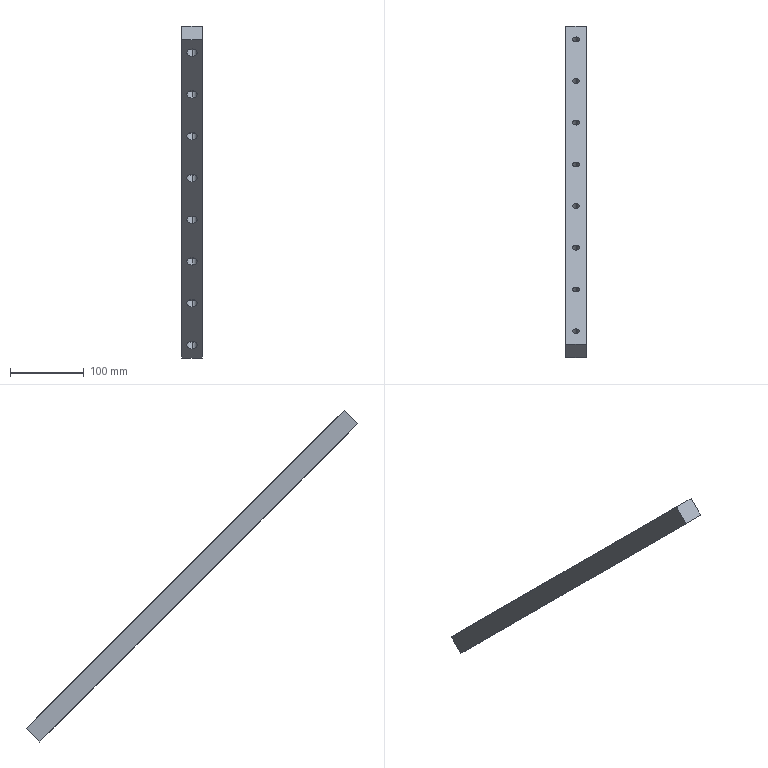Part | STEP file | X-Axis 28 Guide Rail | 1 solid | 46 faces | box 28 x 449.72 x 449.72 mm | volume 422177 mm3 | cylinder 32 | plane 14 | commonest cylinder face diameters 9 x16 14 x16
STEP:
#1=CARTESIAN_POINT('',(-773.,626.059,-470.164));
#2=VERTEX_POINT('',#1);
#3=CARTESIAN_POINT('',(-773.,632.423,-476.527));
#4=VERTEX_POINT('',#3);
#5=CARTESIAN_POINT('',(-773.,629.241,-473.346));
#6=DIRECTION('',(0.,-0.7071,-0.7071));
#7=DIRECTION('',(0.,0.7071,-0.7071));
#8=AXIS2_PLACEMENT_3D('',#5,#6,#7);
#9=CIRCLE('',#8,4.5);
#10=EDGE_CURVE('',#2,#4,#9,.T.);
#11=ORIENTED_EDGE('',*,*,#10,.F.);
#12=CARTESIAN_POINT('',(-773.,616.16,-480.063));
#13=VERTEX_POINT('',#12);
#14=CARTESIAN_POINT('',(-773.,607.674,-488.548));
#15=DIRECTION('',(0.,-0.7071,-0.7071));
#16=VECTOR('',#15,1000.);
#17=LINE('',#14,#16);
#18=EDGE_CURVE('',#2,#13,#17,.T.);
#19=ORIENTED_EDGE('',*,*,#18,.T.);
#20=CARTESIAN_POINT('',(-773.,622.524,-486.427));
#21=VERTEX_POINT('',#20);
#22=CARTESIAN_POINT('',(-773.,619.342,-483.245));
#23=DIRECTION('',(0.,0.7071,0.7071));
#24=DIRECTION('',(0.,0.7071,-0.7071));
#25=AXIS2_PLACEMENT_3D('',#22,#23,#24);
#26=CIRCLE('',#25,4.5);
#27=EDGE_CURVE('',#21,#13,#26,.T.);
#28=ORIENTED_EDGE('',*,*,#27,.F.);
#29=CARTESIAN_POINT('',(-773.,614.038,-494.912));
#30=DIRECTION('',(0.,-0.7071,-0.7071));
#31=VECTOR('',#30,1000.);
#32=LINE('',#29,#31);
#33=EDGE_CURVE('',#4,#21,#32,.T.);
#34=ORIENTED_EDGE('',*,*,#33,.F.);
#35=EDGE_LOOP('',(#11,#19,#28,#34));
#36=FACE_OUTER_BOUND('',#35,.T.);
#37=CARTESIAN_POINT('',(-773.,610.856,-491.73));
#38=DIRECTION('',(0.,-0.7071,-0.7071));
#39=DIRECTION('',(0.,0.7071,-0.7071));
#40=AXIS2_PLACEMENT_3D('',#37,#38,#39);
#41=CYLINDRICAL_SURFACE('',#40,4.5);
#42=ADVANCED_FACE('',(#36),#41,.F.);
#43=CARTESIAN_POINT('',(-773.,682.628,-526.732));
#44=VERTEX_POINT('',#43);
#45=CARTESIAN_POINT('',(-773.,688.992,-533.096));
#46=VERTEX_POINT('',#45);
#47=CARTESIAN_POINT('',(-773.,685.81,-529.914));
#48=DIRECTION('',(0.,-0.7071,-0.7071));
#49=DIRECTION('',(0.,0.7071,-0.7071));
#50=AXIS2_PLACEMENT_3D('',#47,#48,#49);
#51=CIRCLE('',#50,4.5);
#52=EDGE_CURVE('',#44,#46,#51,.T.);
#53=ORIENTED_EDGE('',*,*,#52,.F.);
#54=CARTESIAN_POINT('',(-773.,672.728,-536.632));
#55=VERTEX_POINT('',#54);
#56=CARTESIAN_POINT('',(-773.,664.243,-545.117));
#57=DIRECTION('',(0.,-0.7071,-0.7071));
#58=VECTOR('',#57,1000.);
#59=LINE('',#56,#58);
#60=EDGE_CURVE('',#44,#55,#59,.T.);
#61=ORIENTED_EDGE('',*,*,#60,.T.);
#62=CARTESIAN_POINT('',(-773.,679.092,-542.996));
#63=VERTEX_POINT('',#62);
#64=CARTESIAN_POINT('',(-773.,675.91,-539.814));
#65=DIRECTION('',(0.,0.7071,0.7071));
#66=DIRECTION('',(0.,0.7071,-0.7071));
#67=AXIS2_PLACEMENT_3D('',#64,#65,#66);
#68=CIRCLE('',#67,4.5);
#69=EDGE_CURVE('',#63,#55,#68,.T.);
#70=ORIENTED_EDGE('',*,*,#69,.F.);
#71=CARTESIAN_POINT('',(-773.,670.607,-551.481));
#72=DIRECTION('',(0.,-0.7071,-0.7071));
#73=VECTOR('',#72,1000.);
#74=LINE('',#71,#73);
#75=EDGE_CURVE('',#46,#63,#74,.T.);
#76=ORIENTED_EDGE('',*,*,#75,.F.);
#77=EDGE_LOOP('',(#53,#61,#70,#76));
#78=FACE_OUTER_BOUND('',#77,.T.);
#79=CARTESIAN_POINT('',(-773.,667.425,-548.299));
#80=DIRECTION('',(0.,-0.7071,-0.7071));
#81=DIRECTION('',(0.,0.7071,-0.7071));
#82=AXIS2_PLACEMENT_3D('',#79,#80,#81);
#83=CYLINDRICAL_SURFACE('',#82,4.5);
#84=ADVANCED_FACE('',(#78),#83,.F.);
#85=CARTESIAN_POINT('',(-773.,456.354,-300.458));
#86=VERTEX_POINT('',#85);
#87=CARTESIAN_POINT('',(-773.,462.717,-306.822));
#88=VERTEX_POINT('',#87);
#89=CARTESIAN_POINT('',(-773.,459.536,-303.64));
#90=DIRECTION('',(0.,-0.7071,-0.7071));
#91=DIRECTION('',(0.,0.7071,-0.7071));
#92=AXIS2_PLACEMENT_3D('',#89,#90,#91);
#93=CIRCLE('',#92,4.5);
#94=EDGE_CURVE('',#86,#88,#93,.T.);
#95=ORIENTED_EDGE('',*,*,#94,.F.);
#96=CARTESIAN_POINT('',(-773.,446.454,-310.357));
#97=VERTEX_POINT('',#96);
#98=CARTESIAN_POINT('',(-773.,437.969,-318.843));
#99=DIRECTION('',(0.,-0.7071,-0.7071));
#100=VECTOR('',#99,1000.);
#101=LINE('',#98,#100);
#102=EDGE_CURVE('',#86,#97,#101,.T.);
#103=ORIENTED_EDGE('',*,*,#102,.T.);
#104=CARTESIAN_POINT('',(-773.,452.818,-316.721));
#105=VERTEX_POINT('',#104);
#106=CARTESIAN_POINT('',(-773.,449.636,-313.539));
#107=DIRECTION('',(0.,0.7071,0.7071));
#108=DIRECTION('',(0.,0.7071,-0.7071));
#109=AXIS2_PLACEMENT_3D('',#106,#107,#108);
#110=CIRCLE('',#109,4.5);
#111=EDGE_CURVE('',#105,#97,#110,.T.);
#112=ORIENTED_EDGE('',*,*,#111,.F.);
#113=CARTESIAN_POINT('',(-773.,444.333,-325.207));
#114=DIRECTION('',(0.,-0.7071,-0.7071));
#115=VECTOR('',#114,1000.);
#116=LINE('',#113,#115);
#117=EDGE_CURVE('',#88,#105,#116,.T.);
#118=ORIENTED_EDGE('',*,*,#117,.F.);
#119=EDGE_LOOP('',(#95,#103,#112,#118));
#120=FACE_OUTER_BOUND('',#119,.T.);
#121=CARTESIAN_POINT('',(-773.,441.151,-322.025));
#122=DIRECTION('',(0.,-0.7071,-0.7071));
#123=DIRECTION('',(0.,0.7071,-0.7071));
#124=AXIS2_PLACEMENT_3D('',#121,#122,#123);
#125=CYLINDRICAL_SURFACE('',#124,4.5);
#126=ADVANCED_FACE('',(#120),#125,.F.);
#127=CARTESIAN_POINT('',(-773.,569.491,-413.595));
#128=VERTEX_POINT('',#127);
#129=CARTESIAN_POINT('',(-773.,575.855,-419.959));
#130=VERTEX_POINT('',#129);
#131=CARTESIAN_POINT('',(-773.,572.673,-416.777));
#132=DIRECTION('',(0.,-0.7071,-0.7071));
#133=DIRECTION('',(0.,0.7071,-0.7071));
#134=AXIS2_PLACEMENT_3D('',#131,#132,#133);
#135=CIRCLE('',#134,4.5);
#136=EDGE_CURVE('',#128,#130,#135,.T.);
#137=ORIENTED_EDGE('',*,*,#136,.F.);
#138=CARTESIAN_POINT('',(-773.,559.591,-423.494));
#139=VERTEX_POINT('',#138);
#140=CARTESIAN_POINT('',(-773.,551.106,-431.98));
#141=DIRECTION('',(0.,-0.7071,-0.7071));
#142=VECTOR('',#141,1000.);
#143=LINE('',#140,#142);
#144=EDGE_CURVE('',#128,#139,#143,.T.);
#145=ORIENTED_EDGE('',*,*,#144,.T.);
#146=CARTESIAN_POINT('',(-773.,565.955,-429.858));
#147=VERTEX_POINT('',#146);
#148=CARTESIAN_POINT('',(-773.,562.773,-426.676));
#149=DIRECTION('',(0.,0.7071,0.7071));
#150=DIRECTION('',(0.,0.7071,-0.7071));
#151=AXIS2_PLACEMENT_3D('',#148,#149,#150);
#152=CIRCLE('',#151,4.5);
#153=EDGE_CURVE('',#147,#139,#152,.T.);
#154=ORIENTED_EDGE('',*,*,#153,.F.);
#155=CARTESIAN_POINT('',(-773.,557.47,-438.344));
#156=DIRECTION('',(0.,-0.7071,-0.7071));
#157=VECTOR('',#156,1000.);
#158=LINE('',#155,#157);
#159=EDGE_CURVE('',#130,#147,#158,.T.);
#160=ORIENTED_EDGE('',*,*,#159,.F.);
#161=EDGE_LOOP('',(#137,#145,#154,#160));
#162=FACE_OUTER_BOUND('',#161,.T.);
#163=CARTESIAN_POINT('',(-773.,554.288,-435.162));
#164=DIRECTION('',(0.,-0.7071,-0.7071));
#165=DIRECTION('',(0.,0.7071,-0.7071));
#166=AXIS2_PLACEMENT_3D('',#163,#164,#165);
#167=CYLINDRICAL_SURFACE('',#166,4.5);
#168=ADVANCED_FACE('',(#162),#167,.F.);
#169=CARTESIAN_POINT('',(-773.,512.922,-357.026));
#170=VERTEX_POINT('',#169);
#171=CARTESIAN_POINT('',(-773.,519.286,-363.39));
#172=VERTEX_POINT('',#171);
#173=CARTESIAN_POINT('',(-773.,516.104,-360.208));
#174=DIRECTION('',(0.,-0.7071,-0.7071));
#175=DIRECTION('',(0.,0.7071,-0.7071));
#176=AXIS2_PLACEMENT_3D('',#173,#174,#175);
#177=CIRCLE('',#176,4.5);
#178=EDGE_CURVE('',#170,#172,#177,.T.);
#179=ORIENTED_EDGE('',*,*,#178,.F.);
#180=CARTESIAN_POINT('',(-773.,503.023,-366.926));
#181=VERTEX_POINT('',#180);
#182=CARTESIAN_POINT('',(-773.,494.537,-375.411));
#183=DIRECTION('',(0.,-0.7071,-0.7071));
#184=VECTOR('',#183,1000.);
#185=LINE('',#182,#184);
#186=EDGE_CURVE('',#170,#181,#185,.T.);
#187=ORIENTED_EDGE('',*,*,#186,.T.);
#188=CARTESIAN_POINT('',(-773.,509.387,-373.29));
#189=VERTEX_POINT('',#188);
#190=CARTESIAN_POINT('',(-773.,506.205,-370.108));
#191=DIRECTION('',(0.,0.7071,0.7071));
#192=DIRECTION('',(0.,0.7071,-0.7071));
#193=AXIS2_PLACEMENT_3D('',#190,#191,#192);
#194=CIRCLE('',#193,4.5);
#195=EDGE_CURVE('',#189,#181,#194,.T.);
#196=ORIENTED_EDGE('',*,*,#195,.F.);
#197=CARTESIAN_POINT('',(-773.,500.901,-381.775));
#198=DIRECTION('',(0.,-0.7071,-0.7071));
#199=VECTOR('',#198,1000.);
#200=LINE('',#197,#199);
#201=EDGE_CURVE('',#172,#189,#200,.T.);
#202=ORIENTED_EDGE('',*,*,#201,.F.);
#203=EDGE_LOOP('',(#179,#187,#196,#202));
#204=FACE_OUTER_BOUND('',#203,.T.);
#205=CARTESIAN_POINT('',(-773.,497.719,-378.593));
#206=DIRECTION('',(0.,-0.7071,-0.7071));
#207=DIRECTION('',(0.,0.7071,-0.7071));
#208=AXIS2_PLACEMENT_3D('',#205,#206,#207);
#209=CYLINDRICAL_SURFACE('',#208,4.5);
#210=ADVANCED_FACE('',(#204),#209,.F.);
#211=CARTESIAN_POINT('',(-773.,343.216,-187.321));
#212=VERTEX_POINT('',#211);
#213=CARTESIAN_POINT('',(-773.,349.58,-193.685));
#214=VERTEX_POINT('',#213);
#215=CARTESIAN_POINT('',(-773.,346.398,-190.503));
#216=DIRECTION('',(0.,-0.7071,-0.7071));
#217=DIRECTION('',(0.,0.7071,-0.7071));
#218=AXIS2_PLACEMENT_3D('',#215,#216,#217);
#219=CIRCLE('',#218,4.5);
#220=EDGE_CURVE('',#212,#214,#219,.T.);
#221=ORIENTED_EDGE('',*,*,#220,.F.);
#222=CARTESIAN_POINT('',(-773.,333.317,-197.22));
#223=VERTEX_POINT('',#222);
#224=CARTESIAN_POINT('',(-773.,324.832,-205.706));
#225=DIRECTION('',(0.,-0.7071,-0.7071));
#226=VECTOR('',#225,1000.);
#227=LINE('',#224,#226);
#228=EDGE_CURVE('',#212,#223,#227,.T.);
#229=ORIENTED_EDGE('',*,*,#228,.T.);
#230=CARTESIAN_POINT('',(-773.,339.681,-203.584));
#231=VERTEX_POINT('',#230);
#232=CARTESIAN_POINT('',(-773.,336.499,-200.402));
#233=DIRECTION('',(0.,0.7071,0.7071));
#234=DIRECTION('',(0.,0.7071,-0.7071));
#235=AXIS2_PLACEMENT_3D('',#232,#233,#234);
#236=CIRCLE('',#235,4.5);
#237=EDGE_CURVE('',#231,#223,#236,.T.);
#238=ORIENTED_EDGE('',*,*,#237,.F.);
#239=CARTESIAN_POINT('',(-773.,331.196,-212.07));
#240=DIRECTION('',(0.,-0.7071,-0.7071));
#241=VECTOR('',#240,1000.);
#242=LINE('',#239,#241);
#243=EDGE_CURVE('',#214,#231,#242,.T.);
#244=ORIENTED_EDGE('',*,*,#243,.F.);
#245=EDGE_LOOP('',(#221,#229,#238,#244));
#246=FACE_OUTER_BOUND('',#245,.T.);
#247=CARTESIAN_POINT('',(-773.,328.014,-208.888));
#248=DIRECTION('',(0.,-0.7071,-0.7071));
#249=DIRECTION('',(0.,0.7071,-0.7071));
#250=AXIS2_PLACEMENT_3D('',#247,#248,#249);
#251=CYLINDRICAL_SURFACE('',#250,4.5);
#252=ADVANCED_FACE('',(#246),#251,.F.);
#253=CARTESIAN_POINT('',(-773.,399.785,-243.889));
#254=VERTEX_POINT('',#253);
#255=CARTESIAN_POINT('',(-773.,406.149,-250.253));
#256=VERTEX_POINT('',#255);
#257=CARTESIAN_POINT('',(-773.,402.967,-247.071));
#258=DIRECTION('',(0.,-0.7071,-0.7071));
#259=DIRECTION('',(0.,0.7071,-0.7071));
#260=AXIS2_PLACEMENT_3D('',#257,#258,#259);
#261=CIRCLE('',#260,4.5);
#262=EDGE_CURVE('',#254,#256,#261,.T.);
#263=ORIENTED_EDGE('',*,*,#262,.F.);
#264=CARTESIAN_POINT('',(-773.,389.885,-253.789));
#265=VERTEX_POINT('',#264);
#266=CARTESIAN_POINT('',(-773.,381.4,-262.274));
#267=DIRECTION('',(0.,-0.7071,-0.7071));
#268=VECTOR('',#267,1000.);
#269=LINE('',#266,#268);
#270=EDGE_CURVE('',#254,#265,#269,.T.);
#271=ORIENTED_EDGE('',*,*,#270,.T.);
#272=CARTESIAN_POINT('',(-773.,396.249,-260.153));
#273=VERTEX_POINT('',#272);
#274=CARTESIAN_POINT('',(-773.,393.067,-256.971));
#275=DIRECTION('',(0.,0.7071,0.7071));
#276=DIRECTION('',(0.,0.7071,-0.7071));
#277=AXIS2_PLACEMENT_3D('',#274,#275,#276);
#278=CIRCLE('',#277,4.5);
#279=EDGE_CURVE('',#273,#265,#278,.T.);
#280=ORIENTED_EDGE('',*,*,#279,.F.);
#281=CARTESIAN_POINT('',(-773.,387.764,-268.638));
#282=DIRECTION('',(0.,-0.7071,-0.7071));
#283=VECTOR('',#282,1000.);
#284=LINE('',#281,#283);
#285=EDGE_CURVE('',#256,#273,#284,.T.);
#286=ORIENTED_EDGE('',*,*,#285,.F.);
#287=EDGE_LOOP('',(#263,#271,#280,#286));
#288=FACE_OUTER_BOUND('',#287,.T.);
#289=CARTESIAN_POINT('',(-773.,384.582,-265.456));
#290=DIRECTION('',(0.,-0.7071,-0.7071));
#291=DIRECTION('',(0.,0.7071,-0.7071));
#292=AXIS2_PLACEMENT_3D('',#289,#290,#291);
#293=CYLINDRICAL_SURFACE('',#292,4.5);
#294=ADVANCED_FACE('',(#288),#293,.F.);
#295=CARTESIAN_POINT('',(-773.,286.648,-130.752));
#296=VERTEX_POINT('',#295);
#297=CARTESIAN_POINT('',(-773.,293.012,-137.116));
#298=VERTEX_POINT('',#297);
#299=CARTESIAN_POINT('',(-773.,289.83,-133.934));
#300=DIRECTION('',(0.,-0.7071,-0.7071));
#301=DIRECTION('',(0.,0.7071,-0.7071));
#302=AXIS2_PLACEMENT_3D('',#299,#300,#301);
#303=CIRCLE('',#302,4.5);
#304=EDGE_CURVE('',#296,#298,#303,.T.);
#305=ORIENTED_EDGE('',*,*,#304,.F.);
#306=CARTESIAN_POINT('',(-773.,276.748,-140.652));
#307=VERTEX_POINT('',#306);
#308=CARTESIAN_POINT('',(-773.,268.263,-149.137));
#309=DIRECTION('',(0.,-0.7071,-0.7071));
#310=VECTOR('',#309,1000.);
#311=LINE('',#308,#310);
#312=EDGE_CURVE('',#296,#307,#311,.T.);
#313=ORIENTED_EDGE('',*,*,#312,.T.);
#314=CARTESIAN_POINT('',(-773.,283.112,-147.016));
#315=VERTEX_POINT('',#314);
#316=CARTESIAN_POINT('',(-773.,279.93,-143.834));
#317=DIRECTION('',(0.,0.7071,0.7071));
#318=DIRECTION('',(0.,0.7071,-0.7071));
#319=AXIS2_PLACEMENT_3D('',#316,#317,#318);
#320=CIRCLE('',#319,4.5);
#321=EDGE_CURVE('',#315,#307,#320,.T.);
#322=ORIENTED_EDGE('',*,*,#321,.F.);
#323=CARTESIAN_POINT('',(-773.,274.627,-155.501));
#324=DIRECTION('',(0.,-0.7071,-0.7071));
#325=VECTOR('',#324,1000.);
#326=LINE('',#323,#325);
#327=EDGE_CURVE('',#298,#315,#326,.T.);
#328=ORIENTED_EDGE('',*,*,#327,.F.);
#329=EDGE_LOOP('',(#305,#313,#322,#328));
#330=FACE_OUTER_BOUND('',#329,.T.);
#331=CARTESIAN_POINT('',(-773.,271.445,-152.319));
#332=DIRECTION('',(0.,-0.7071,-0.7071));
#333=DIRECTION('',(0.,0.7071,-0.7071));
#334=AXIS2_PLACEMENT_3D('',#331,#332,#333);
#335=CYLINDRICAL_SURFACE('',#334,4.5);
#336=ADVANCED_FACE('',(#330),#335,.F.);
#337=CARTESIAN_POINT('',(-773.,624.291,-488.195));
#338=VERTEX_POINT('',#337);
#339=CARTESIAN_POINT('',(-773.,614.392,-478.295));
#340=VERTEX_POINT('',#339);
#341=CARTESIAN_POINT('',(-773.,619.342,-483.245));
#342=DIRECTION('',(0.,0.7071,0.7071));
#343=DIRECTION('',(0.,0.7071,-0.7071));
#344=AXIS2_PLACEMENT_3D('',#341,#342,#343);
#345=CIRCLE('',#344,7.);
#346=EDGE_CURVE('',#338,#340,#345,.T.);
#347=ORIENTED_EDGE('',*,*,#346,.T.);
#348=CARTESIAN_POINT('',(-773.,605.907,-486.781));
#349=VERTEX_POINT('',#348);
#350=CARTESIAN_POINT('',(-773.,605.907,-486.781));
#351=DIRECTION('',(0.,-0.7071,-0.7071));
#352=VECTOR('',#351,1000.);
#353=LINE('',#350,#352);
#354=EDGE_CURVE('',#340,#349,#353,.T.);
#355=ORIENTED_EDGE('',*,*,#354,.T.);
#356=CARTESIAN_POINT('',(-773.,615.806,-496.68));
#357=VERTEX_POINT('',#356);
#358=CARTESIAN_POINT('',(-773.,610.856,-491.73));
#359=DIRECTION('',(0.,-0.7071,-0.7071));
#360=DIRECTION('',(0.,0.7071,-0.7071));
#361=AXIS2_PLACEMENT_3D('',#358,#359,#360);
#362=CIRCLE('',#361,7.);
#363=EDGE_CURVE('',#349,#357,#362,.T.);
#364=ORIENTED_EDGE('',*,*,#363,.T.);
#365=CARTESIAN_POINT('',(-773.,615.806,-496.68));
#366=DIRECTION('',(0.,-0.7071,-0.7071));
#367=VECTOR('',#366,1000.);
#368=LINE('',#365,#367);
#369=EDGE_CURVE('',#338,#357,#368,.T.);
#370=ORIENTED_EDGE('',*,*,#369,.F.);
#371=EDGE_LOOP('',(#347,#355,#364,#370));
#372=FACE_OUTER_BOUND('',#371,.T.);
#373=CARTESIAN_POINT('',(-773.,610.856,-491.73));
#374=DIRECTION('',(0.,-0.7071,-0.7071));
#375=DIRECTION('',(0.,0.7071,-0.7071));
#376=AXIS2_PLACEMENT_3D('',#373,#374,#375);
#377=CYLINDRICAL_SURFACE('',#376,7.);
#378=ADVANCED_FACE('',(#372),#377,.F.);
#379=CARTESIAN_POINT('',(-773.,680.86,-544.763));
#380=VERTEX_POINT('',#379);
#381=CARTESIAN_POINT('',(-773.,670.96,-534.864));
#382=VERTEX_POINT('',#381);
#383=CARTESIAN_POINT('',(-773.,675.91,-539.814));
#384=DIRECTION('',(0.,0.7071,0.7071));
#385=DIRECTION('',(0.,0.7071,-0.7071));
#386=AXIS2_PLACEMENT_3D('',#383,#384,#385);
#387=CIRCLE('',#386,7.);
#388=EDGE_CURVE('',#380,#382,#387,.T.);
#389=ORIENTED_EDGE('',*,*,#388,.T.);
#390=CARTESIAN_POINT('',(-773.,662.475,-543.349));
#391=VERTEX_POINT('',#390);
#392=CARTESIAN_POINT('',(-773.,662.475,-543.349));
#393=DIRECTION('',(0.,-0.7071,-0.7071));
#394=VECTOR('',#393,1000.);
#395=LINE('',#392,#394);
#396=EDGE_CURVE('',#382,#391,#395,.T.);
#397=ORIENTED_EDGE('',*,*,#396,.T.);
#398=CARTESIAN_POINT('',(-773.,672.375,-553.249));
#399=VERTEX_POINT('',#398);
#400=CARTESIAN_POINT('',(-773.,667.425,-548.299));
#401=DIRECTION('',(0.,-0.7071,-0.7071));
#402=DIRECTION('',(0.,0.7071,-0.7071));
#403=AXIS2_PLACEMENT_3D('',#400,#401,#402);
#404=CIRCLE('',#403,7.);
#405=EDGE_CURVE('',#391,#399,#404,.T.);
#406=ORIENTED_EDGE('',*,*,#405,.T.);
#407=CARTESIAN_POINT('',(-773.,672.375,-553.249));
#408=DIRECTION('',(0.,-0.7071,-0.7071));
#409=VECTOR('',#408,1000.);
#410=LINE('',#407,#409);
#411=EDGE_CURVE('',#380,#399,#410,.T.);
#412=ORIENTED_EDGE('',*,*,#411,.F.);
#413=EDGE_LOOP('',(#389,#397,#406,#412));
#414=FACE_OUTER_BOUND('',#413,.T.);
#415=CARTESIAN_POINT('',(-773.,667.425,-548.299));
#416=DIRECTION('',(0.,-0.7071,-0.7071));
#417=DIRECTION('',(0.,0.7071,-0.7071));
#418=AXIS2_PLACEMENT_3D('',#415,#416,#417);
#419=CYLINDRICAL_SURFACE('',#418,7.);
#420=ADVANCED_FACE('',(#414),#419,.F.);
#421=CARTESIAN_POINT('',(-773.,454.586,-318.489));
#422=VERTEX_POINT('',#421);
#423=CARTESIAN_POINT('',(-773.,444.686,-308.59));
#424=VERTEX_POINT('',#423);
#425=CARTESIAN_POINT('',(-773.,449.636,-313.539));
#426=DIRECTION('',(0.,0.7071,0.7071));
#427=DIRECTION('',(0.,0.7071,-0.7071));
#428=AXIS2_PLACEMENT_3D('',#425,#426,#427);
#429=CIRCLE('',#428,7.);
#430=EDGE_CURVE('',#422,#424,#429,.T.);
#431=ORIENTED_EDGE('',*,*,#430,.T.);
#432=CARTESIAN_POINT('',(-773.,436.201,-317.075));
#433=VERTEX_POINT('',#432);
#434=CARTESIAN_POINT('',(-773.,436.201,-317.075));
#435=DIRECTION('',(0.,-0.7071,-0.7071));
#436=VECTOR('',#435,1000.);
#437=LINE('',#434,#436);
#438=EDGE_CURVE('',#424,#433,#437,.T.);
#439=ORIENTED_EDGE('',*,*,#438,.T.);
#440=CARTESIAN_POINT('',(-773.,446.1,-326.974));
#441=VERTEX_POINT('',#440);
#442=CARTESIAN_POINT('',(-773.,441.151,-322.025));
#443=DIRECTION('',(0.,-0.7071,-0.7071));
#444=DIRECTION('',(0.,0.7071,-0.7071));
#445=AXIS2_PLACEMENT_3D('',#442,#443,#444);
#446=CIRCLE('',#445,7.);
#447=EDGE_CURVE('',#433,#441,#446,.T.);
#448=ORIENTED_EDGE('',*,*,#447,.T.);
#449=CARTESIAN_POINT('',(-773.,446.1,-326.974));
#450=DIRECTION('',(0.,-0.7071,-0.7071));
#451=VECTOR('',#450,1000.);
#452=LINE('',#449,#451);
#453=EDGE_CURVE('',#422,#441,#452,.T.);
#454=ORIENTED_EDGE('',*,*,#453,.F.);
#455=EDGE_LOOP('',(#431,#439,#448,#454));
#456=FACE_OUTER_BOUND('',#455,.T.);
#457=CARTESIAN_POINT('',(-773.,441.151,-322.025));
#458=DIRECTION('',(0.,-0.7071,-0.7071));
#459=DIRECTION('',(0.,0.7071,-0.7071));
#460=AXIS2_PLACEMENT_3D('',#457,#458,#459);
#461=CYLINDRICAL_SURFACE('',#460,7.);
#462=ADVANCED_FACE('',(#456),#461,.F.);
#463=CARTESIAN_POINT('',(-773.,567.723,-431.626));
#464=VERTEX_POINT('',#463);
#465=CARTESIAN_POINT('',(-773.,557.823,-421.727));
#466=VERTEX_POINT('',#465);
#467=CARTESIAN_POINT('',(-773.,562.773,-426.676));
#468=DIRECTION('',(0.,0.7071,0.7071));
#469=DIRECTION('',(0.,0.7071,-0.7071));
#470=AXIS2_PLACEMENT_3D('',#467,#468,#469);
#471=CIRCLE('',#470,7.);
#472=EDGE_CURVE('',#464,#466,#471,.T.);
#473=ORIENTED_EDGE('',*,*,#472,.T.);
#474=CARTESIAN_POINT('',(-773.,549.338,-430.212));
#475=VERTEX_POINT('',#474);
#476=CARTESIAN_POINT('',(-773.,549.338,-430.212));
#477=DIRECTION('',(0.,-0.7071,-0.7071));
#478=VECTOR('',#477,1000.);
#479=LINE('',#476,#478);
#480=EDGE_CURVE('',#466,#475,#479,.T.);
#481=ORIENTED_EDGE('',*,*,#480,.T.);
#482=CARTESIAN_POINT('',(-773.,559.238,-440.111));
#483=VERTEX_POINT('',#482);
#484=CARTESIAN_POINT('',(-773.,554.288,-435.162));
#485=DIRECTION('',(0.,-0.7071,-0.7071));
#486=DIRECTION('',(0.,0.7071,-0.7071));
#487=AXIS2_PLACEMENT_3D('',#484,#485,#486);
#488=CIRCLE('',#487,7.);
#489=EDGE_CURVE('',#475,#483,#488,.T.);
#490=ORIENTED_EDGE('',*,*,#489,.T.);
#491=CARTESIAN_POINT('',(-773.,559.238,-440.111));
#492=DIRECTION('',(0.,-0.7071,-0.7071));
#493=VECTOR('',#492,1000.);
#494=LINE('',#491,#493);
#495=EDGE_CURVE('',#464,#483,#494,.T.);
#496=ORIENTED_EDGE('',*,*,#495,.F.);
#497=EDGE_LOOP('',(#473,#481,#490,#496));
#498=FACE_OUTER_BOUND('',#497,.T.);
#499=CARTESIAN_POINT('',(-773.,554.288,-435.162));
#500=DIRECTION('',(0.,-0.7071,-0.7071));
#501=DIRECTION('',(0.,0.7071,-0.7071));
#502=AXIS2_PLACEMENT_3D('',#499,#500,#501);
#503=CYLINDRICAL_SURFACE('',#502,7.);
#504=ADVANCED_FACE('',(#498),#503,.F.);
#505=CARTESIAN_POINT('',(-773.,511.154,-375.058));
#506=VERTEX_POINT('',#505);
#507=CARTESIAN_POINT('',(-773.,501.255,-365.158));
#508=VERTEX_POINT('',#507);
#509=CARTESIAN_POINT('',(-773.,506.205,-370.108));
#510=DIRECTION('',(0.,0.7071,0.7071));
#511=DIRECTION('',(0.,0.7071,-0.7071));
#512=AXIS2_PLACEMENT_3D('',#509,#510,#511);
#513=CIRCLE('',#512,7.);
#514=EDGE_CURVE('',#506,#508,#513,.T.);
#515=ORIENTED_EDGE('',*,*,#514,.T.);
#516=CARTESIAN_POINT('',(-773.,492.77,-373.643));
#517=VERTEX_POINT('',#516);
#518=CARTESIAN_POINT('',(-773.,492.77,-373.643));
#519=DIRECTION('',(0.,-0.7071,-0.7071));
#520=VECTOR('',#519,1000.);
#521=LINE('',#518,#520);
#522=EDGE_CURVE('',#508,#517,#521,.T.);
#523=ORIENTED_EDGE('',*,*,#522,.T.);
#524=CARTESIAN_POINT('',(-773.,502.669,-383.543));
#525=VERTEX_POINT('',#524);
#526=CARTESIAN_POINT('',(-773.,497.719,-378.593));
#527=DIRECTION('',(0.,-0.7071,-0.7071));
#528=DIRECTION('',(0.,0.7071,-0.7071));
#529=AXIS2_PLACEMENT_3D('',#526,#527,#528);
#530=CIRCLE('',#529,7.);
#531=EDGE_CURVE('',#517,#525,#530,.T.);
#532=ORIENTED_EDGE('',*,*,#531,.T.);
#533=CARTESIAN_POINT('',(-773.,502.669,-383.543));
#534=DIRECTION('',(0.,-0.7071,-0.7071));
#535=VECTOR('',#534,1000.);
#536=LINE('',#533,#535);
#537=EDGE_CURVE('',#506,#525,#536,.T.);
#538=ORIENTED_EDGE('',*,*,#537,.F.);
#539=EDGE_LOOP('',(#515,#523,#532,#538));
#540=FACE_OUTER_BOUND('',#539,.T.);
#541=CARTESIAN_POINT('',(-773.,497.719,-378.593));
#542=DIRECTION('',(0.,-0.7071,-0.7071));
#543=DIRECTION('',(0.,0.7071,-0.7071));
#544=AXIS2_PLACEMENT_3D('',#541,#542,#543);
#545=CYLINDRICAL_SURFACE('',#544,7.);
#546=ADVANCED_FACE('',(#540),#545,.F.);
#547=CARTESIAN_POINT('',(-773.,341.449,-205.352));
#548=VERTEX_POINT('',#547);
#549=CARTESIAN_POINT('',(-773.,331.549,-195.453));
#550=VERTEX_POINT('',#549);
#551=CARTESIAN_POINT('',(-773.,336.499,-200.402));
#552=DIRECTION('',(0.,0.7071,0.7071));
#553=DIRECTION('',(0.,0.7071,-0.7071));
#554=AXIS2_PLACEMENT_3D('',#551,#552,#553);
#555=CIRCLE('',#554,7.);
#556=EDGE_CURVE('',#548,#550,#555,.T.);
#557=ORIENTED_EDGE('',*,*,#556,.T.);
#558=CARTESIAN_POINT('',(-773.,323.064,-203.938));
#559=VERTEX_POINT('',#558);
#560=CARTESIAN_POINT('',(-773.,323.064,-203.938));
#561=DIRECTION('',(0.,-0.7071,-0.7071));
#562=VECTOR('',#561,1000.);
#563=LINE('',#560,#562);
#564=EDGE_CURVE('',#550,#559,#563,.T.);
#565=ORIENTED_EDGE('',*,*,#564,.T.);
#566=CARTESIAN_POINT('',(-773.,332.963,-213.837));
#567=VERTEX_POINT('',#566);
#568=CARTESIAN_POINT('',(-773.,328.014,-208.888));
#569=DIRECTION('',(0.,-0.7071,-0.7071));
#570=DIRECTION('',(0.,0.7071,-0.7071));
#571=AXIS2_PLACEMENT_3D('',#568,#569,#570);
#572=CIRCLE('',#571,7.);
#573=EDGE_CURVE('',#559,#567,#572,.T.);
#574=ORIENTED_EDGE('',*,*,#573,.T.);
#575=CARTESIAN_POINT('',(-773.,332.963,-213.837));
#576=DIRECTION('',(0.,-0.7071,-0.7071));
#577=VECTOR('',#576,1000.);
#578=LINE('',#575,#577);
#579=EDGE_CURVE('',#548,#567,#578,.T.);
#580=ORIENTED_EDGE('',*,*,#579,.F.);
#581=EDGE_LOOP('',(#557,#565,#574,#580));
#582=FACE_OUTER_BOUND('',#581,.T.);
#583=CARTESIAN_POINT('',(-773.,328.014,-208.888));
#584=DIRECTION('',(0.,-0.7071,-0.7071));
#585=DIRECTION('',(0.,0.7071,-0.7071));
#586=AXIS2_PLACEMENT_3D('',#583,#584,#585);
#587=CYLINDRICAL_SURFACE('',#586,7.);
#588=ADVANCED_FACE('',(#582),#587,.F.);
#589=CARTESIAN_POINT('',(-773.,398.017,-261.921));
#590=VERTEX_POINT('',#589);
#591=CARTESIAN_POINT('',(-773.,388.118,-252.021));
#592=VERTEX_POINT('',#591);
#593=CARTESIAN_POINT('',(-773.,393.067,-256.971));
#594=DIRECTION('',(0.,0.7071,0.7071));
#595=DIRECTION('',(0.,0.7071,-0.7071));
#596=AXIS2_PLACEMENT_3D('',#593,#594,#595);
#597=CIRCLE('',#596,7.);
#598=EDGE_CURVE('',#590,#592,#597,.T.);
#599=ORIENTED_EDGE('',*,*,#598,.T.);
#600=CARTESIAN_POINT('',(-773.,379.632,-260.506));
#601=VERTEX_POINT('',#600);
#602=CARTESIAN_POINT('',(-773.,379.632,-260.506));
#603=DIRECTION('',(0.,-0.7071,-0.7071));
#604=VECTOR('',#603,1000.);
#605=LINE('',#602,#604);
#606=EDGE_CURVE('',#592,#601,#605,.T.);
#607=ORIENTED_EDGE('',*,*,#606,.T.);
#608=CARTESIAN_POINT('',(-773.,389.532,-270.406));
#609=VERTEX_POINT('',#608);
#610=CARTESIAN_POINT('',(-773.,384.582,-265.456));
#611=DIRECTION('',(0.,-0.7071,-0.7071));
#612=DIRECTION('',(0.,0.7071,-0.7071));
#613=AXIS2_PLACEMENT_3D('',#610,#611,#612);
#614=CIRCLE('',#613,7.);
#615=EDGE_CURVE('',#601,#609,#614,.T.);
#616=ORIENTED_EDGE('',*,*,#615,.T.);
#617=CARTESIAN_POINT('',(-773.,389.532,-270.406));
#618=DIRECTION('',(0.,-0.7071,-0.7071));
#619=VECTOR('',#618,1000.);
#620=LINE('',#617,#619);
#621=EDGE_CURVE('',#590,#609,#620,.T.);
#622=ORIENTED_EDGE('',*,*,#621,.F.);
#623=EDGE_LOOP('',(#599,#607,#616,#622));
#624=FACE_OUTER_BOUND('',#623,.T.);
#625=CARTESIAN_POINT('',(-773.,384.582,-265.456));
#626=DIRECTION('',(0.,-0.7071,-0.7071));
#627=DIRECTION('',(0.,0.7071,-0.7071));
#628=AXIS2_PLACEMENT_3D('',#625,#626,#627);
#629=CYLINDRICAL_SURFACE('',#628,7.);
#630=ADVANCED_FACE('',(#624),#629,.F.);
#631=CARTESIAN_POINT('',(-773.,284.88,-148.783));
#632=VERTEX_POINT('',#631);
#633=CARTESIAN_POINT('',(-773.,274.981,-138.884));
#634=VERTEX_POINT('',#633);
#635=CARTESIAN_POINT('',(-773.,279.93,-143.834));
#636=DIRECTION('',(0.,0.7071,0.7071));
#637=DIRECTION('',(0.,0.7071,-0.7071));
#638=AXIS2_PLACEMENT_3D('',#635,#636,#637);
#639=CIRCLE('',#638,7.);
#640=EDGE_CURVE('',#632,#634,#639,.T.);
#641=ORIENTED_EDGE('',*,*,#640,.T.);
#642=CARTESIAN_POINT('',(-773.,266.495,-147.369));
#643=VERTEX_POINT('',#642);
#644=CARTESIAN_POINT('',(-773.,266.495,-147.369));
#645=DIRECTION('',(0.,-0.7071,-0.7071));
#646=VECTOR('',#645,1000.);
#647=LINE('',#644,#646);
#648=EDGE_CURVE('',#634,#643,#647,.T.);
#649=ORIENTED_EDGE('',*,*,#648,.T.);
#650=CARTESIAN_POINT('',(-773.,276.395,-157.269));
#651=VERTEX_POINT('',#650);
#652=CARTESIAN_POINT('',(-773.,271.445,-152.319));
#653=DIRECTION('',(0.,-0.7071,-0.7071));
#654=DIRECTION('',(0.,0.7071,-0.7071));
#655=AXIS2_PLACEMENT_3D('',#652,#653,#654);
#656=CIRCLE('',#655,7.);
#657=EDGE_CURVE('',#643,#651,#656,.T.);
#658=ORIENTED_EDGE('',*,*,#657,.T.);
#659=CARTESIAN_POINT('',(-773.,276.395,-157.269));
#660=DIRECTION('',(0.,-0.7071,-0.7071));
#661=VECTOR('',#660,1000.);
#662=LINE('',#659,#661);
#663=EDGE_CURVE('',#632,#651,#662,.T.);
#664=ORIENTED_EDGE('',*,*,#663,.F.);
#665=EDGE_LOOP('',(#641,#649,#658,#664));
#666=FACE_OUTER_BOUND('',#665,.T.);
#667=CARTESIAN_POINT('',(-773.,271.445,-152.319));
#668=DIRECTION('',(0.,-0.7071,-0.7071));
#669=DIRECTION('',(0.,0.7071,-0.7071));
#670=AXIS2_PLACEMENT_3D('',#667,#668,#669);
#671=CYLINDRICAL_SURFACE('',#670,7.);
#672=ADVANCED_FACE('',(#666),#671,.F.);
#673=CARTESIAN_POINT('',(-759.,703.487,-547.592));
#674=VERTEX_POINT('',#673);
#675=CARTESIAN_POINT('',(-787.,703.487,-547.592));
#676=VERTEX_POINT('',#675);
#677=CARTESIAN_POINT('',(0.,703.487,-547.592));
#678=DIRECTION('',(-1.,0.,0.));
#679=VECTOR('',#678,1000.);
#680=LINE('',#677,#679);
#681=EDGE_CURVE('',#674,#676,#680,.T.);
#682=ORIENTED_EDGE('',*,*,#681,.T.);
#683=CARTESIAN_POINT('',(-787.,272.152,-116.257));
#684=VERTEX_POINT('',#683);
#685=CARTESIAN_POINT('',(-787.,77.948,77.948));
#686=DIRECTION('',(0.,-0.7071,0.7071));
#687=VECTOR('',#686,1000.);
#688=LINE('',#685,#687);
#689=EDGE_CURVE('',#676,#684,#688,.T.);
#690=ORIENTED_EDGE('',*,*,#689,.T.);
#691=CARTESIAN_POINT('',(-759.,272.152,-116.257));
#692=VERTEX_POINT('',#691);
#693=CARTESIAN_POINT('',(0.,272.152,-116.257));
#694=DIRECTION('',(1.,0.,0.));
#695=VECTOR('',#694,1000.);
#696=LINE('',#693,#695);
#697=EDGE_CURVE('',#684,#692,#696,.T.);
#698=ORIENTED_EDGE('',*,*,#697,.T.);
#699=CARTESIAN_POINT('',(-759.,77.948,77.948));
#700=DIRECTION('',(0.,0.7071,-0.7071));
#701=VECTOR('',#700,1000.);
#702=LINE('',#699,#701);
#703=EDGE_CURVE('',#692,#674,#702,.T.);
#704=ORIENTED_EDGE('',*,*,#703,.T.);
#705=EDGE_LOOP('',(#682,#690,#698,#704));
#706=FACE_OUTER_BOUND('',#705,.T.);
#707=CARTESIAN_POINT('',(-773.,629.241,-473.346));
#708=DIRECTION('',(0.,-0.7071,-0.7071));
#709=DIRECTION('',(0.,0.7071,-0.7071));
#710=AXIS2_PLACEMENT_3D('',#707,#708,#709);
#711=CIRCLE('',#710,4.5);
#712=EDGE_CURVE('',#4,#2,#711,.T.);
#713=ORIENTED_EDGE('',*,*,#712,.T.);
#714=ORIENTED_EDGE('',*,*,#10,.T.);
#715=EDGE_LOOP('',(#713,#714));
#716=FACE_BOUND('',#715,.T.);
#717=CARTESIAN_POINT('',(-773.,685.81,-529.914));
#718=DIRECTION('',(0.,-0.7071,-0.7071));
#719=DIRECTION('',(0.,0.7071,-0.7071));
#720=AXIS2_PLACEMENT_3D('',#717,#718,#719);
#721=CIRCLE('',#720,4.5);
#722=EDGE_CURVE('',#46,#44,#721,.T.);
#723=ORIENTED_EDGE('',*,*,#722,.T.);
#724=ORIENTED_EDGE('',*,*,#52,.T.);
#725=EDGE_LOOP('',(#723,#724));
#726=FACE_BOUND('',#725,.T.);
#727=CARTESIAN_POINT('',(-773.,459.536,-303.64));
#728=DIRECTION('',(0.,-0.7071,-0.7071));
#729=DIRECTION('',(0.,0.7071,-0.7071));
#730=AXIS2_PLACEMENT_3D('',#727,#728,#729);
#731=CIRCLE('',#730,4.5);
#732=EDGE_CURVE('',#88,#86,#731,.T.);
#733=ORIENTED_EDGE('',*,*,#732,.T.);
#734=ORIENTED_EDGE('',*,*,#94,.T.);
#735=EDGE_LOOP('',(#733,#734));
#736=FACE_BOUND('',#735,.T.);
#737=CARTESIAN_POINT('',(-773.,572.673,-416.777));
#738=DIRECTION('',(0.,-0.7071,-0.7071));
#739=DIRECTION('',(0.,0.7071,-0.7071));
#740=AXIS2_PLACEMENT_3D('',#737,#738,#739);
#741=CIRCLE('',#740,4.5);
#742=EDGE_CURVE('',#130,#128,#741,.T.);
#743=ORIENTED_EDGE('',*,*,#742,.T.);
#744=ORIENTED_EDGE('',*,*,#136,.T.);
#745=EDGE_LOOP('',(#743,#744));
#746=FACE_BOUND('',#745,.T.);
#747=CARTESIAN_POINT('',(-773.,516.104,-360.208));
#748=DIRECTION('',(0.,-0.7071,-0.7071));
#749=DIRECTION('',(0.,0.7071,-0.7071));
#750=AXIS2_PLACEMENT_3D('',#747,#748,#749);
#751=CIRCLE('',#750,4.5);
#752=EDGE_CURVE('',#172,#170,#751,.T.);
#753=ORIENTED_EDGE('',*,*,#752,.T.);
#754=ORIENTED_EDGE('',*,*,#178,.T.);
#755=EDGE_LOOP('',(#753,#754));
#756=FACE_BOUND('',#755,.T.);
#757=CARTESIAN_POINT('',(-773.,346.398,-190.503));
#758=DIRECTION('',(0.,-0.7071,-0.7071));
#759=DIRECTION('',(0.,0.7071,-0.7071));
#760=AXIS2_PLACEMENT_3D('',#757,#758,#759);
#761=CIRCLE('',#760,4.5);
#762=EDGE_CURVE('',#214,#212,#761,.T.);
#763=ORIENTED_EDGE('',*,*,#762,.T.);
#764=ORIENTED_EDGE('',*,*,#220,.T.);
#765=EDGE_LOOP('',(#763,#764));
#766=FACE_BOUND('',#765,.T.);
#767=CARTESIAN_POINT('',(-773.,402.967,-247.071));
#768=DIRECTION('',(0.,-0.7071,-0.7071));
#769=DIRECTION('',(0.,0.7071,-0.7071));
#770=AXIS2_PLACEMENT_3D('',#767,#768,#769);
#771=CIRCLE('',#770,4.5);
#772=EDGE_CURVE('',#256,#254,#771,.T.);
#773=ORIENTED_EDGE('',*,*,#772,.T.);
#774=ORIENTED_EDGE('',*,*,#262,.T.);
#775=EDGE_LOOP('',(#773,#774));
#776=FACE_BOUND('',#775,.T.);
#777=CARTESIAN_POINT('',(-773.,289.83,-133.934));
#778=DIRECTION('',(0.,-0.7071,-0.7071));
#779=DIRECTION('',(0.,0.7071,-0.7071));
#780=AXIS2_PLACEMENT_3D('',#777,#778,#779);
#781=CIRCLE('',#780,4.5);
#782=EDGE_CURVE('',#298,#296,#781,.T.);
#783=ORIENTED_EDGE('',*,*,#782,.T.);
#784=ORIENTED_EDGE('',*,*,#304,.T.);
#785=EDGE_LOOP('',(#783,#784));
#786=FACE_BOUND('',#785,.T.);
#787=CARTESIAN_POINT('',(0.,77.948,77.948));
#788=DIRECTION('',(0.,0.7071,0.7071));
#789=DIRECTION('',(0.,-0.7071,0.7071));
#790=AXIS2_PLACEMENT_3D('',#787,#788,#789);
#791=PLANE('',#790);
#792=ADVANCED_FACE('',(#706,#716,#726,#736,#746,#756,#766,#776,#786),#791,.T.);
#793=CARTESIAN_POINT('',(-787.,685.103,-565.977));
#794=VERTEX_POINT('',#793);
#795=CARTESIAN_POINT('',(-787.,253.767,-134.641));
#796=VERTEX_POINT('',#795);
#797=CARTESIAN_POINT('',(-787.,685.103,-565.977));
#798=DIRECTION('',(0.,-0.7071,0.7071));
#799=VECTOR('',#798,1000.);
#800=LINE('',#797,#799);
#801=EDGE_CURVE('',#794,#796,#800,.T.);
#802=ORIENTED_EDGE('',*,*,#801,.T.);
#803=CARTESIAN_POINT('',(-787.,253.767,-134.641));
#804=DIRECTION('',(0.,0.7071,0.7071));
#805=VECTOR('',#804,1000.);
#806=LINE('',#803,#805);
#807=EDGE_CURVE('',#796,#684,#806,.T.);
#808=ORIENTED_EDGE('',*,*,#807,.T.);
#809=ORIENTED_EDGE('',*,*,#689,.F.);
#810=CARTESIAN_POINT('',(-787.,703.487,-547.592));
#811=DIRECTION('',(0.,-0.7071,-0.7071));
#812=VECTOR('',#811,1000.);
#813=LINE('',#810,#812);
#814=EDGE_CURVE('',#676,#794,#813,.T.);
#815=ORIENTED_EDGE('',*,*,#814,.T.);
#816=EDGE_LOOP('',(#802,#808,#809,#815));
#817=FACE_OUTER_BOUND('',#816,.T.);
#818=CARTESIAN_POINT('',(-787.,685.103,-565.977));
#819=DIRECTION('',(-1.,0.,0.));
#820=DIRECTION('',(0.,0.,1.));
#821=AXIS2_PLACEMENT_3D('',#818,#819,#820);
#822=PLANE('',#821);
#823=ADVANCED_FACE('',(#817),#822,.T.);
#824=CARTESIAN_POINT('',(-759.,685.103,-565.977));
#825=VERTEX_POINT('',#824);
#826=CARTESIAN_POINT('',(-759.,685.103,-565.977));
#827=DIRECTION('',(-1.,0.,0.));
#828=VECTOR('',#827,1000.);
#829=LINE('',#826,#828);
#830=EDGE_CURVE('',#825,#794,#829,.T.);
#831=ORIENTED_EDGE('',*,*,#830,.T.);
#832=ORIENTED_EDGE('',*,*,#814,.F.);
#833=ORIENTED_EDGE('',*,*,#681,.F.);
#834=CARTESIAN_POINT('',(-759.,685.103,-565.977));
#835=DIRECTION('',(0.,-0.7071,-0.7071));
#836=VECTOR('',#835,1000.);
#837=LINE('',#834,#836);
#838=EDGE_CURVE('',#674,#825,#837,.T.);
#839=ORIENTED_EDGE('',*,*,#838,.T.);
#840=EDGE_LOOP('',(#831,#832,#833,#839));
#841=FACE_OUTER_BOUND('',#840,.T.);
#842=CARTESIAN_POINT('',(-759.,685.103,-565.977));
#843=DIRECTION('',(0.,0.7071,-0.7071));
#844=DIRECTION('',(0.,0.7071,0.7071));
#845=AXIS2_PLACEMENT_3D('',#842,#843,#844);
#846=PLANE('',#845);
#847=ADVANCED_FACE('',(#841),#846,.T.);
#848=CARTESIAN_POINT('',(-759.,253.767,-134.641));
#849=VERTEX_POINT('',#848);
#850=CARTESIAN_POINT('',(-759.,253.767,-134.641));
#851=DIRECTION('',(0.,0.7071,-0.7071));
#852=VECTOR('',#851,1000.);
#853=LINE('',#850,#852);
#854=EDGE_CURVE('',#849,#825,#853,.T.);
#855=ORIENTED_EDGE('',*,*,#854,.T.);
#856=ORIENTED_EDGE('',*,*,#838,.F.);
#857=ORIENTED_EDGE('',*,*,#703,.F.);
#858=CARTESIAN_POINT('',(-759.,272.152,-116.257));
#859=DIRECTION('',(0.,-0.7071,-0.7071));
#860=VECTOR('',#859,1000.);
#861=LINE('',#858,#860);
#862=EDGE_CURVE('',#692,#849,#861,.T.);
#863=ORIENTED_EDGE('',*,*,#862,.T.);
#864=EDGE_LOOP('',(#855,#856,#857,#863));
#865=FACE_OUTER_BOUND('',#864,.T.);
#866=CARTESIAN_POINT('',(-759.,253.767,-134.641));
#867=DIRECTION('',(1.,0.,0.));
#868=DIRECTION('',(0.,0.,-1.));
#869=AXIS2_PLACEMENT_3D('',#866,#867,#868);
#870=PLANE('',#869);
#871=ADVANCED_FACE('',(#865),#870,.T.);
#872=CARTESIAN_POINT('',(-787.,253.767,-134.641));
#873=DIRECTION('',(1.,0.,0.));
#874=VECTOR('',#873,1000.);
#875=LINE('',#872,#874);
#876=EDGE_CURVE('',#796,#849,#875,.T.);
#877=ORIENTED_EDGE('',*,*,#876,.T.);
#878=ORIENTED_EDGE('',*,*,#862,.F.);
#879=ORIENTED_EDGE('',*,*,#697,.F.);
#880=ORIENTED_EDGE('',*,*,#807,.F.);
#881=EDGE_LOOP('',(#877,#878,#879,#880));
#882=FACE_OUTER_BOUND('',#881,.T.);
#883=CARTESIAN_POINT('',(-787.,253.767,-134.641));
#884=DIRECTION('',(0.,-0.7071,0.7071));
#885=DIRECTION('',(0.,-0.7071,-0.7071));
#886=AXIS2_PLACEMENT_3D('',#883,#884,#885);
#887=PLANE('',#886);
#888=ADVANCED_FACE('',(#882),#887,.T.);
#889=ORIENTED_EDGE('',*,*,#18,.F.);
#890=ORIENTED_EDGE('',*,*,#712,.F.);
#891=ORIENTED_EDGE('',*,*,#33,.T.);
#892=CARTESIAN_POINT('',(-773.,619.342,-483.245));
#893=DIRECTION('',(0.,0.7071,0.7071));
#894=DIRECTION('',(0.,0.7071,-0.7071));
#895=AXIS2_PLACEMENT_3D('',#892,#893,#894);
#896=CIRCLE('',#895,4.5);
#897=EDGE_CURVE('',#13,#21,#896,.T.);
#898=ORIENTED_EDGE('',*,*,#897,.F.);
#899=EDGE_LOOP('',(#889,#890,#891,#898));
#900=FACE_OUTER_BOUND('',#899,.T.);
#901=CARTESIAN_POINT('',(-773.,610.856,-491.73));
#902=DIRECTION('',(0.,-0.7071,-0.7071));
#903=DIRECTION('',(0.,0.7071,-0.7071));
#904=AXIS2_PLACEMENT_3D('',#901,#902,#903);
#905=CYLINDRICAL_SURFACE('',#904,4.5);
#906=ADVANCED_FACE('',(#900),#905,.F.);
#907=ORIENTED_EDGE('',*,*,#60,.F.);
#908=ORIENTED_EDGE('',*,*,#722,.F.);
#909=ORIENTED_EDGE('',*,*,#75,.T.);
#910=CARTESIAN_POINT('',(-773.,675.91,-539.814));
#911=DIRECTION('',(0.,0.7071,0.7071));
#912=DIRECTION('',(0.,0.7071,-0.7071));
#913=AXIS2_PLACEMENT_3D('',#910,#911,#912);
#914=CIRCLE('',#913,4.5);
#915=EDGE_CURVE('',#55,#63,#914,.T.);
#916=ORIENTED_EDGE('',*,*,#915,.F.);
#917=EDGE_LOOP('',(#907,#908,#909,#916));
#918=FACE_OUTER_BOUND('',#917,.T.);
#919=CARTESIAN_POINT('',(-773.,667.425,-548.299));
#920=DIRECTION('',(0.,-0.7071,-0.7071));
#921=DIRECTION('',(0.,0.7071,-0.7071));
#922=AXIS2_PLACEMENT_3D('',#919,#920,#921);
#923=CYLINDRICAL_SURFACE('',#922,4.5);
#924=ADVANCED_FACE('',(#918),#923,.F.);
#925=ORIENTED_EDGE('',*,*,#102,.F.);
#926=ORIENTED_EDGE('',*,*,#732,.F.);
#927=ORIENTED_EDGE('',*,*,#117,.T.);
#928=CARTESIAN_POINT('',(-773.,449.636,-313.539));
#929=DIRECTION('',(0.,0.7071,0.7071));
#930=DIRECTION('',(0.,0.7071,-0.7071));
#931=AXIS2_PLACEMENT_3D('',#928,#929,#930);
#932=CIRCLE('',#931,4.5);
#933=EDGE_CURVE('',#97,#105,#932,.T.);
#934=ORIENTED_EDGE('',*,*,#933,.F.);
#935=EDGE_LOOP('',(#925,#926,#927,#934));
#936=FACE_OUTER_BOUND('',#935,.T.);
#937=CARTESIAN_POINT('',(-773.,441.151,-322.025));
#938=DIRECTION('',(0.,-0.7071,-0.7071));
#939=DIRECTION('',(0.,0.7071,-0.7071));
#940=AXIS2_PLACEMENT_3D('',#937,#938,#939);
#941=CYLINDRICAL_SURFACE('',#940,4.5);
#942=ADVANCED_FACE('',(#936),#941,.F.);
#943=ORIENTED_EDGE('',*,*,#144,.F.);
#944=ORIENTED_EDGE('',*,*,#742,.F.);
#945=ORIENTED_EDGE('',*,*,#159,.T.);
#946=CARTESIAN_POINT('',(-773.,562.773,-426.676));
#947=DIRECTION('',(0.,0.7071,0.7071));
#948=DIRECTION('',(0.,0.7071,-0.7071));
#949=AXIS2_PLACEMENT_3D('',#946,#947,#948);
#950=CIRCLE('',#949,4.5);
#951=EDGE_CURVE('',#139,#147,#950,.T.);
#952=ORIENTED_EDGE('',*,*,#951,.F.);
#953=EDGE_LOOP('',(#943,#944,#945,#952));
#954=FACE_OUTER_BOUND('',#953,.T.);
#955=CARTESIAN_POINT('',(-773.,554.288,-435.162));
#956=DIRECTION('',(0.,-0.7071,-0.7071));
#957=DIRECTION('',(0.,0.7071,-0.7071));
#958=AXIS2_PLACEMENT_3D('',#955,#956,#957);
#959=CYLINDRICAL_SURFACE('',#958,4.5);
#960=ADVANCED_FACE('',(#954),#959,.F.);
#961=ORIENTED_EDGE('',*,*,#186,.F.);
#962=ORIENTED_EDGE('',*,*,#752,.F.);
#963=ORIENTED_EDGE('',*,*,#201,.T.);
#964=CARTESIAN_POINT('',(-773.,506.205,-370.108));
#965=DIRECTION('',(0.,0.7071,0.7071));
#966=DIRECTION('',(0.,0.7071,-0.7071));
#967=AXIS2_PLACEMENT_3D('',#964,#965,#966);
#968=CIRCLE('',#967,4.5);
#969=EDGE_CURVE('',#181,#189,#968,.T.);
#970=ORIENTED_EDGE('',*,*,#969,.F.);
#971=EDGE_LOOP('',(#961,#962,#963,#970));
#972=FACE_OUTER_BOUND('',#971,.T.);
#973=CARTESIAN_POINT('',(-773.,497.719,-378.593));
#974=DIRECTION('',(0.,-0.7071,-0.7071));
#975=DIRECTION('',(0.,0.7071,-0.7071));
#976=AXIS2_PLACEMENT_3D('',#973,#974,#975);
#977=CYLINDRICAL_SURFACE('',#976,4.5);
#978=ADVANCED_FACE('',(#972),#977,.F.);
#979=ORIENTED_EDGE('',*,*,#228,.F.);
#980=ORIENTED_EDGE('',*,*,#762,.F.);
#981=ORIENTED_EDGE('',*,*,#243,.T.);
#982=CARTESIAN_POINT('',(-773.,336.499,-200.402));
#983=DIRECTION('',(0.,0.7071,0.7071));
#984=DIRECTION('',(0.,0.7071,-0.7071));
#985=AXIS2_PLACEMENT_3D('',#982,#983,#984);
#986=CIRCLE('',#985,4.5);
#987=EDGE_CURVE('',#223,#231,#986,.T.);
#988=ORIENTED_EDGE('',*,*,#987,.F.);
#989=EDGE_LOOP('',(#979,#980,#981,#988));
#990=FACE_OUTER_BOUND('',#989,.T.);
#991=CARTESIAN_POINT('',(-773.,328.014,-208.888));
#992=DIRECTION('',(0.,-0.7071,-0.7071));
#993=DIRECTION('',(0.,0.7071,-0.7071));
#994=AXIS2_PLACEMENT_3D('',#991,#992,#993);
#995=CYLINDRICAL_SURFACE('',#994,4.5);
#996=ADVANCED_FACE('',(#990),#995,.F.);
#997=ORIENTED_EDGE('',*,*,#270,.F.);
#998=ORIENTED_EDGE('',*,*,#772,.F.);
#999=ORIENTED_EDGE('',*,*,#285,.T.);
#1000=CARTESIAN_POINT('',(-773.,393.067,-256.971));
#1001=DIRECTION('',(0.,0.7071,0.7071));
#1002=DIRECTION('',(0.,0.7071,-0.7071));
#1003=AXIS2_PLACEMENT_3D('',#1000,#1001,#1002);
#1004=CIRCLE('',#1003,4.5);
#1005=EDGE_CURVE('',#265,#273,#1004,.T.);
#1006=ORIENTED_EDGE('',*,*,#1005,.F.);
#1007=EDGE_LOOP('',(#997,#998,#999,#1006));
#1008=FACE_OUTER_BOUND('',#1007,.T.);
#1009=CARTESIAN_POINT('',(-773.,384.582,-265.456));
#1010=DIRECTION('',(0.,-0.7071,-0.7071));
#1011=DIRECTION('',(0.,0.7071,-0.7071));
#1012=AXIS2_PLACEMENT_3D('',#1009,#1010,#1011);
#1013=CYLINDRICAL_SURFACE('',#1012,4.5);
#1014=ADVANCED_FACE('',(#1008),#1013,.F.);
#1015=ORIENTED_EDGE('',*,*,#312,.F.);
#1016=ORIENTED_EDGE('',*,*,#782,.F.);
#1017=ORIENTED_EDGE('',*,*,#327,.T.);
#1018=CARTESIAN_POINT('',(-773.,279.93,-143.834));
#1019=DIRECTION('',(0.,0.7071,0.7071));
#1020=DIRECTION('',(0.,0.7071,-0.7071));
#1021=AXIS2_PLACEMENT_3D('',#1018,#1019,#1020);
#1022=CIRCLE('',#1021,4.5);
#1023=EDGE_CURVE('',#307,#315,#1022,.T.);
#1024=ORIENTED_EDGE('',*,*,#1023,.F.);
#1025=EDGE_LOOP('',(#1015,#1016,#1017,#1024));
#1026=FACE_OUTER_BOUND('',#1025,.T.);
#1027=CARTESIAN_POINT('',(-773.,271.445,-152.319));
#1028=DIRECTION('',(0.,-0.7071,-0.7071));
#1029=DIRECTION('',(0.,0.7071,-0.7071));
#1030=AXIS2_PLACEMENT_3D('',#1027,#1028,#1029);
#1031=CYLINDRICAL_SURFACE('',#1030,4.5);
#1032=ADVANCED_FACE('',(#1026),#1031,.F.);
#1033=ORIENTED_EDGE('',*,*,#801,.F.);
#1034=ORIENTED_EDGE('',*,*,#830,.F.);
#1035=ORIENTED_EDGE('',*,*,#854,.F.);
#1036=ORIENTED_EDGE('',*,*,#876,.F.);
#1037=EDGE_LOOP('',(#1033,#1034,#1035,#1036));
#1038=FACE_OUTER_BOUND('',#1037,.T.);
#1039=CARTESIAN_POINT('',(-773.,610.856,-491.73));
#1040=DIRECTION('',(0.,-0.7071,-0.7071));
#1041=DIRECTION('',(0.,0.7071,-0.7071));
#1042=AXIS2_PLACEMENT_3D('',#1039,#1040,#1041);
#1043=CIRCLE('',#1042,7.);
#1044=EDGE_CURVE('',#357,#349,#1043,.T.);
#1045=ORIENTED_EDGE('',*,*,#1044,.F.);
#1046=ORIENTED_EDGE('',*,*,#363,.F.);
#1047=EDGE_LOOP('',(#1045,#1046));
#1048=FACE_BOUND('',#1047,.T.);
#1049=CARTESIAN_POINT('',(-773.,667.425,-548.299));
#1050=DIRECTION('',(0.,-0.7071,-0.7071));
#1051=DIRECTION('',(0.,0.7071,-0.7071));
#1052=AXIS2_PLACEMENT_3D('',#1049,#1050,#1051);
#1053=CIRCLE('',#1052,7.);
#1054=EDGE_CURVE('',#399,#391,#1053,.T.);
#1055=ORIENTED_EDGE('',*,*,#1054,.F.);
#1056=ORIENTED_EDGE('',*,*,#405,.F.);
#1057=EDGE_LOOP('',(#1055,#1056));
#1058=FACE_BOUND('',#1057,.T.);
#1059=CARTESIAN_POINT('',(-773.,441.151,-322.025));
#1060=DIRECTION('',(0.,-0.7071,-0.7071));
#1061=DIRECTION('',(0.,0.7071,-0.7071));
#1062=AXIS2_PLACEMENT_3D('',#1059,#1060,#1061);
#1063=CIRCLE('',#1062,7.);
#1064=EDGE_CURVE('',#441,#433,#1063,.T.);
#1065=ORIENTED_EDGE('',*,*,#1064,.F.);
#1066=ORIENTED_EDGE('',*,*,#447,.F.);
#1067=EDGE_LOOP('',(#1065,#1066));
#1068=FACE_BOUND('',#1067,.T.);
#1069=CARTESIAN_POINT('',(-773.,554.288,-435.162));
#1070=DIRECTION('',(0.,-0.7071,-0.7071));
#1071=DIRECTION('',(0.,0.7071,-0.7071));
#1072=AXIS2_PLACEMENT_3D('',#1069,#1070,#1071);
#1073=CIRCLE('',#1072,7.);
#1074=EDGE_CURVE('',#483,#475,#1073,.T.);
#1075=ORIENTED_EDGE('',*,*,#1074,.F.);
#1076=ORIENTED_EDGE('',*,*,#489,.F.);
#1077=EDGE_LOOP('',(#1075,#1076));
#1078=FACE_BOUND('',#1077,.T.);
#1079=CARTESIAN_POINT('',(-773.,497.719,-378.593));
#1080=DIRECTION('',(0.,-0.7071,-0.7071));
#1081=DIRECTION('',(0.,0.7071,-0.7071));
#1082=AXIS2_PLACEMENT_3D('',#1079,#1080,#1081);
#1083=CIRCLE('',#1082,7.);
#1084=EDGE_CURVE('',#525,#517,#1083,.T.);
#1085=ORIENTED_EDGE('',*,*,#1084,.F.);
#1086=ORIENTED_EDGE('',*,*,#531,.F.);
#1087=EDGE_LOOP('',(#1085,#1086));
#1088=FACE_BOUND('',#1087,.T.);
#1089=CARTESIAN_POINT('',(-773.,328.014,-208.888));
#1090=DIRECTION('',(0.,-0.7071,-0.7071));
#1091=DIRECTION('',(0.,0.7071,-0.7071));
#1092=AXIS2_PLACEMENT_3D('',#1089,#1090,#1091);
#1093=CIRCLE('',#1092,7.);
#1094=EDGE_CURVE('',#567,#559,#1093,.T.);
#1095=ORIENTED_EDGE('',*,*,#1094,.F.);
#1096=ORIENTED_EDGE('',*,*,#573,.F.);
#1097=EDGE_LOOP('',(#1095,#1096));
#1098=FACE_BOUND('',#1097,.T.);
#1099=CARTESIAN_POINT('',(-773.,384.582,-265.456));
#1100=DIRECTION('',(0.,-0.7071,-0.7071));
#1101=DIRECTION('',(0.,0.7071,-0.7071));
#1102=AXIS2_PLACEMENT_3D('',#1099,#1100,#1101);
#1103=CIRCLE('',#1102,7.);
#1104=EDGE_CURVE('',#609,#601,#1103,.T.);
#1105=ORIENTED_EDGE('',*,*,#1104,.F.);
#1106=ORIENTED_EDGE('',*,*,#615,.F.);
#1107=EDGE_LOOP('',(#1105,#1106));
#1108=FACE_BOUND('',#1107,.T.);
#1109=CARTESIAN_POINT('',(-773.,271.445,-152.319));
#1110=DIRECTION('',(0.,-0.7071,-0.7071));
#1111=DIRECTION('',(0.,0.7071,-0.7071));
#1112=AXIS2_PLACEMENT_3D('',#1109,#1110,#1111);
#1113=CIRCLE('',#1112,7.);
#1114=EDGE_CURVE('',#651,#643,#1113,.T.);
#1115=ORIENTED_EDGE('',*,*,#1114,.F.);
#1116=ORIENTED_EDGE('',*,*,#657,.F.);
#1117=EDGE_LOOP('',(#1115,#1116));
#1118=FACE_BOUND('',#1117,.T.);
#1119=CARTESIAN_POINT('',(0.,59.563,59.563));
#1120=DIRECTION('',(0.,0.7071,0.7071));
#1121=DIRECTION('',(0.,-0.7071,0.7071));
#1122=AXIS2_PLACEMENT_3D('',#1119,#1120,#1121);
#1123=PLANE('',#1122);
#1124=ADVANCED_FACE('',(#1038,#1048,#1058,#1068,#1078,#1088,#1098,#1108,#1118),#1123,.F.);
#1125=ORIENTED_EDGE('',*,*,#346,.F.);
#1126=CARTESIAN_POINT('',(-773.,619.342,-483.245));
#1127=DIRECTION('',(0.,0.7071,0.7071));
#1128=DIRECTION('',(0.,0.7071,-0.7071));
#1129=AXIS2_PLACEMENT_3D('',#1126,#1127,#1128);
#1130=CIRCLE('',#1129,7.);
#1131=EDGE_CURVE('',#340,#338,#1130,.T.);
#1132=ORIENTED_EDGE('',*,*,#1131,.F.);
#1133=EDGE_LOOP('',(#1125,#1132));
#1134=FACE_OUTER_BOUND('',#1133,.T.);
#1135=ORIENTED_EDGE('',*,*,#27,.T.);
#1136=ORIENTED_EDGE('',*,*,#897,.T.);
#1137=EDGE_LOOP('',(#1135,#1136));
#1138=FACE_BOUND('',#1137,.T.);
#1139=CARTESIAN_POINT('',(-768.5,619.342,-483.245));
#1140=DIRECTION('',(0.,0.7071,0.7071));
#1141=DIRECTION('',(0.,-0.7071,0.7071));
#1142=AXIS2_PLACEMENT_3D('',#1139,#1140,#1141);
#1143=PLANE('',#1142);
#1144=ADVANCED_FACE('',(#1134,#1138),#1143,.F.);
#1145=ORIENTED_EDGE('',*,*,#388,.F.);
#1146=CARTESIAN_POINT('',(-773.,675.91,-539.814));
#1147=DIRECTION('',(0.,0.7071,0.7071));
#1148=DIRECTION('',(0.,0.7071,-0.7071));
#1149=AXIS2_PLACEMENT_3D('',#1146,#1147,#1148);
#1150=CIRCLE('',#1149,7.);
#1151=EDGE_CURVE('',#382,#380,#1150,.T.);
#1152=ORIENTED_EDGE('',*,*,#1151,.F.);
#1153=EDGE_LOOP('',(#1145,#1152));
#1154=FACE_OUTER_BOUND('',#1153,.T.);
#1155=ORIENTED_EDGE('',*,*,#69,.T.);
#1156=ORIENTED_EDGE('',*,*,#915,.T.);
#1157=EDGE_LOOP('',(#1155,#1156));
#1158=FACE_BOUND('',#1157,.T.);
#1159=CARTESIAN_POINT('',(-768.5,675.91,-539.814));
#1160=DIRECTION('',(0.,0.7071,0.7071));
#1161=DIRECTION('',(0.,-0.7071,0.7071));
#1162=AXIS2_PLACEMENT_3D('',#1159,#1160,#1161);
#1163=PLANE('',#1162);
#1164=ADVANCED_FACE('',(#1154,#1158),#1163,.F.);
#1165=ORIENTED_EDGE('',*,*,#430,.F.);
#1166=CARTESIAN_POINT('',(-773.,449.636,-313.539));
#1167=DIRECTION('',(0.,0.7071,0.7071));
#1168=DIRECTION('',(0.,0.7071,-0.7071));
#1169=AXIS2_PLACEMENT_3D('',#1166,#1167,#1168);
#1170=CIRCLE('',#1169,7.);
#1171=EDGE_CURVE('',#424,#422,#1170,.T.);
#1172=ORIENTED_EDGE('',*,*,#1171,.F.);
#1173=EDGE_LOOP('',(#1165,#1172));
#1174=FACE_OUTER_BOUND('',#1173,.T.);
#1175=ORIENTED_EDGE('',*,*,#111,.T.);
#1176=ORIENTED_EDGE('',*,*,#933,.T.);
#1177=EDGE_LOOP('',(#1175,#1176));
#1178=FACE_BOUND('',#1177,.T.);
#1179=CARTESIAN_POINT('',(-768.5,449.636,-313.539));
#1180=DIRECTION('',(0.,0.7071,0.7071));
#1181=DIRECTION('',(0.,-0.7071,0.7071));
#1182=AXIS2_PLACEMENT_3D('',#1179,#1180,#1181);
#1183=PLANE('',#1182);
#1184=ADVANCED_FACE('',(#1174,#1178),#1183,.F.);
#1185=ORIENTED_EDGE('',*,*,#472,.F.);
#1186=CARTESIAN_POINT('',(-773.,562.773,-426.676));
#1187=DIRECTION('',(0.,0.7071,0.7071));
#1188=DIRECTION('',(0.,0.7071,-0.7071));
#1189=AXIS2_PLACEMENT_3D('',#1186,#1187,#1188);
#1190=CIRCLE('',#1189,7.);
#1191=EDGE_CURVE('',#466,#464,#1190,.T.);
#1192=ORIENTED_EDGE('',*,*,#1191,.F.);
#1193=EDGE_LOOP('',(#1185,#1192));
#1194=FACE_OUTER_BOUND('',#1193,.T.);
#1195=ORIENTED_EDGE('',*,*,#153,.T.);
#1196=ORIENTED_EDGE('',*,*,#951,.T.);
#1197=EDGE_LOOP('',(#1195,#1196));
#1198=FACE_BOUND('',#1197,.T.);
#1199=CARTESIAN_POINT('',(-768.5,562.773,-426.676));
#1200=DIRECTION('',(0.,0.7071,0.7071));
#1201=DIRECTION('',(0.,-0.7071,0.7071));
#1202=AXIS2_PLACEMENT_3D('',#1199,#1200,#1201);
#1203=PLANE('',#1202);
#1204=ADVANCED_FACE('',(#1194,#1198),#1203,.F.);
#1205=ORIENTED_EDGE('',*,*,#514,.F.);
#1206=CARTESIAN_POINT('',(-773.,506.205,-370.108));
#1207=DIRECTION('',(0.,0.7071,0.7071));
#1208=DIRECTION('',(0.,0.7071,-0.7071));
#1209=AXIS2_PLACEMENT_3D('',#1206,#1207,#1208);
#1210=CIRCLE('',#1209,7.);
#1211=EDGE_CURVE('',#508,#506,#1210,.T.);
#1212=ORIENTED_EDGE('',*,*,#1211,.F.);
#1213=EDGE_LOOP('',(#1205,#1212));
#1214=FACE_OUTER_BOUND('',#1213,.T.);
#1215=ORIENTED_EDGE('',*,*,#195,.T.);
#1216=ORIENTED_EDGE('',*,*,#969,.T.);
#1217=EDGE_LOOP('',(#1215,#1216));
#1218=FACE_BOUND('',#1217,.T.);
#1219=CARTESIAN_POINT('',(-768.5,506.205,-370.108));
#1220=DIRECTION('',(0.,0.7071,0.7071));
#1221=DIRECTION('',(0.,-0.7071,0.7071));
#1222=AXIS2_PLACEMENT_3D('',#1219,#1220,#1221);
#1223=PLANE('',#1222);
#1224=ADVANCED_FACE('',(#1214,#1218),#1223,.F.);
#1225=ORIENTED_EDGE('',*,*,#556,.F.);
#1226=CARTESIAN_POINT('',(-773.,336.499,-200.402));
#1227=DIRECTION('',(0.,0.7071,0.7071));
#1228=DIRECTION('',(0.,0.7071,-0.7071));
#1229=AXIS2_PLACEMENT_3D('',#1226,#1227,#1228);
#1230=CIRCLE('',#1229,7.);
#1231=EDGE_CURVE('',#550,#548,#1230,.T.);
#1232=ORIENTED_EDGE('',*,*,#1231,.F.);
#1233=EDGE_LOOP('',(#1225,#1232));
#1234=FACE_OUTER_BOUND('',#1233,.T.);
#1235=ORIENTED_EDGE('',*,*,#237,.T.);
#1236=ORIENTED_EDGE('',*,*,#987,.T.);
#1237=EDGE_LOOP('',(#1235,#1236));
#1238=FACE_BOUND('',#1237,.T.);
#1239=CARTESIAN_POINT('',(-768.5,336.499,-200.402));
#1240=DIRECTION('',(0.,0.7071,0.7071));
#1241=DIRECTION('',(0.,-0.7071,0.7071));
#1242=AXIS2_PLACEMENT_3D('',#1239,#1240,#1241);
#1243=PLANE('',#1242);
#1244=ADVANCED_FACE('',(#1234,#1238),#1243,.F.);
#1245=ORIENTED_EDGE('',*,*,#598,.F.);
#1246=CARTESIAN_POINT('',(-773.,393.067,-256.971));
#1247=DIRECTION('',(0.,0.7071,0.7071));
#1248=DIRECTION('',(0.,0.7071,-0.7071));
#1249=AXIS2_PLACEMENT_3D('',#1246,#1247,#1248);
#1250=CIRCLE('',#1249,7.);
#1251=EDGE_CURVE('',#592,#590,#1250,.T.);
#1252=ORIENTED_EDGE('',*,*,#1251,.F.);
#1253=EDGE_LOOP('',(#1245,#1252));
#1254=FACE_OUTER_BOUND('',#1253,.T.);
#1255=ORIENTED_EDGE('',*,*,#279,.T.);
#1256=ORIENTED_EDGE('',*,*,#1005,.T.);
#1257=EDGE_LOOP('',(#1255,#1256));
#1258=FACE_BOUND('',#1257,.T.);
#1259=CARTESIAN_POINT('',(-768.5,393.067,-256.971));
#1260=DIRECTION('',(0.,0.7071,0.7071));
#1261=DIRECTION('',(0.,-0.7071,0.7071));
#1262=AXIS2_PLACEMENT_3D('',#1259,#1260,#1261);
#1263=PLANE('',#1262);
#1264=ADVANCED_FACE('',(#1254,#1258),#1263,.F.);
#1265=ORIENTED_EDGE('',*,*,#640,.F.);
#1266=CARTESIAN_POINT('',(-773.,279.93,-143.834));
#1267=DIRECTION('',(0.,0.7071,0.7071));
#1268=DIRECTION('',(0.,0.7071,-0.7071));
#1269=AXIS2_PLACEMENT_3D('',#1266,#1267,#1268);
#1270=CIRCLE('',#1269,7.);
#1271=EDGE_CURVE('',#634,#632,#1270,.T.);
#1272=ORIENTED_EDGE('',*,*,#1271,.F.);
#1273=EDGE_LOOP('',(#1265,#1272));
#1274=FACE_OUTER_BOUND('',#1273,.T.);
#1275=ORIENTED_EDGE('',*,*,#321,.T.);
#1276=ORIENTED_EDGE('',*,*,#1023,.T.);
#1277=EDGE_LOOP('',(#1275,#1276));
#1278=FACE_BOUND('',#1277,.T.);
#1279=CARTESIAN_POINT('',(-768.5,279.93,-143.834));
#1280=DIRECTION('',(0.,0.7071,0.7071));
#1281=DIRECTION('',(0.,-0.7071,0.7071));
#1282=AXIS2_PLACEMENT_3D('',#1279,#1280,#1281);
#1283=PLANE('',#1282);
#1284=ADVANCED_FACE('',(#1274,#1278),#1283,.F.);
#1285=ORIENTED_EDGE('',*,*,#354,.F.);
#1286=ORIENTED_EDGE('',*,*,#1131,.T.);
#1287=ORIENTED_EDGE('',*,*,#369,.T.);
#1288=ORIENTED_EDGE('',*,*,#1044,.T.);
#1289=EDGE_LOOP('',(#1285,#1286,#1287,#1288));
#1290=FACE_OUTER_BOUND('',#1289,.T.);
#1291=CARTESIAN_POINT('',(-773.,610.856,-491.73));
#1292=DIRECTION('',(0.,-0.7071,-0.7071));
#1293=DIRECTION('',(0.,0.7071,-0.7071));
#1294=AXIS2_PLACEMENT_3D('',#1291,#1292,#1293);
#1295=CYLINDRICAL_SURFACE('',#1294,7.);
#1296=ADVANCED_FACE('',(#1290),#1295,.F.);
#1297=ORIENTED_EDGE('',*,*,#396,.F.);
#1298=ORIENTED_EDGE('',*,*,#1151,.T.);
#1299=ORIENTED_EDGE('',*,*,#411,.T.);
#1300=ORIENTED_EDGE('',*,*,#1054,.T.);
#1301=EDGE_LOOP('',(#1297,#1298,#1299,#1300));
#1302=FACE_OUTER_BOUND('',#1301,.T.);
#1303=CARTESIAN_POINT('',(-773.,667.425,-548.299));
#1304=DIRECTION('',(0.,-0.7071,-0.7071));
#1305=DIRECTION('',(0.,0.7071,-0.7071));
#1306=AXIS2_PLACEMENT_3D('',#1303,#1304,#1305);
#1307=CYLINDRICAL_SURFACE('',#1306,7.);
#1308=ADVANCED_FACE('',(#1302),#1307,.F.);
#1309=ORIENTED_EDGE('',*,*,#438,.F.);
#1310=ORIENTED_EDGE('',*,*,#1171,.T.);
#1311=ORIENTED_EDGE('',*,*,#453,.T.);
#1312=ORIENTED_EDGE('',*,*,#1064,.T.);
#1313=EDGE_LOOP('',(#1309,#1310,#1311,#1312));
#1314=FACE_OUTER_BOUND('',#1313,.T.);
#1315=CARTESIAN_POINT('',(-773.,441.151,-322.025));
#1316=DIRECTION('',(0.,-0.7071,-0.7071));
#1317=DIRECTION('',(0.,0.7071,-0.7071));
#1318=AXIS2_PLACEMENT_3D('',#1315,#1316,#1317);
#1319=CYLINDRICAL_SURFACE('',#1318,7.);
#1320=ADVANCED_FACE('',(#1314),#1319,.F.);
#1321=ORIENTED_EDGE('',*,*,#480,.F.);
#1322=ORIENTED_EDGE('',*,*,#1191,.T.);
#1323=ORIENTED_EDGE('',*,*,#495,.T.);
#1324=ORIENTED_EDGE('',*,*,#1074,.T.);
#1325=EDGE_LOOP('',(#1321,#1322,#1323,#1324));
#1326=FACE_OUTER_BOUND('',#1325,.T.);
#1327=CARTESIAN_POINT('',(-773.,554.288,-435.162));
#1328=DIRECTION('',(0.,-0.7071,-0.7071));
#1329=DIRECTION('',(0.,0.7071,-0.7071));
#1330=AXIS2_PLACEMENT_3D('',#1327,#1328,#1329);
#1331=CYLINDRICAL_SURFACE('',#1330,7.);
#1332=ADVANCED_FACE('',(#1326),#1331,.F.);
#1333=ORIENTED_EDGE('',*,*,#522,.F.);
#1334=ORIENTED_EDGE('',*,*,#1211,.T.);
#1335=ORIENTED_EDGE('',*,*,#537,.T.);
#1336=ORIENTED_EDGE('',*,*,#1084,.T.);
#1337=EDGE_LOOP('',(#1333,#1334,#1335,#1336));
#1338=FACE_OUTER_BOUND('',#1337,.T.);
#1339=CARTESIAN_POINT('',(-773.,497.719,-378.593));
#1340=DIRECTION('',(0.,-0.7071,-0.7071));
#1341=DIRECTION('',(0.,0.7071,-0.7071));
#1342=AXIS2_PLACEMENT_3D('',#1339,#1340,#1341);
#1343=CYLINDRICAL_SURFACE('',#1342,7.);
#1344=ADVANCED_FACE('',(#1338),#1343,.F.);
#1345=ORIENTED_EDGE('',*,*,#564,.F.);
#1346=ORIENTED_EDGE('',*,*,#1231,.T.);
#1347=ORIENTED_EDGE('',*,*,#579,.T.);
#1348=ORIENTED_EDGE('',*,*,#1094,.T.);
#1349=EDGE_LOOP('',(#1345,#1346,#1347,#1348));
#1350=FACE_OUTER_BOUND('',#1349,.T.);
#1351=CARTESIAN_POINT('',(-773.,328.014,-208.888));
#1352=DIRECTION('',(0.,-0.7071,-0.7071));
#1353=DIRECTION('',(0.,0.7071,-0.7071));
#1354=AXIS2_PLACEMENT_3D('',#1351,#1352,#1353);
#1355=CYLINDRICAL_SURFACE('',#1354,7.);
#1356=ADVANCED_FACE('',(#1350),#1355,.F.);
#1357=ORIENTED_EDGE('',*,*,#606,.F.);
#1358=ORIENTED_EDGE('',*,*,#1251,.T.);
#1359=ORIENTED_EDGE('',*,*,#621,.T.);
#1360=ORIENTED_EDGE('',*,*,#1104,.T.);
#1361=EDGE_LOOP('',(#1357,#1358,#1359,#1360));
#1362=FACE_OUTER_BOUND('',#1361,.T.);
#1363=CARTESIAN_POINT('',(-773.,384.582,-265.456));
#1364=DIRECTION('',(0.,-0.7071,-0.7071));
#1365=DIRECTION('',(0.,0.7071,-0.7071));
#1366=AXIS2_PLACEMENT_3D('',#1363,#1364,#1365);
#1367=CYLINDRICAL_SURFACE('',#1366,7.);
#1368=ADVANCED_FACE('',(#1362),#1367,.F.);
#1369=ORIENTED_EDGE('',*,*,#648,.F.);
#1370=ORIENTED_EDGE('',*,*,#1271,.T.);
#1371=ORIENTED_EDGE('',*,*,#663,.T.);
#1372=ORIENTED_EDGE('',*,*,#1114,.T.);
#1373=EDGE_LOOP('',(#1369,#1370,#1371,#1372));
#1374=FACE_OUTER_BOUND('',#1373,.T.);
#1375=CARTESIAN_POINT('',(-773.,271.445,-152.319));
#1376=DIRECTION('',(0.,-0.7071,-0.7071));
#1377=DIRECTION('',(0.,0.7071,-0.7071));
#1378=AXIS2_PLACEMENT_3D('',#1375,#1376,#1377);
#1379=CYLINDRICAL_SURFACE('',#1378,7.);
#1380=ADVANCED_FACE('',(#1374),#1379,.F.);
#1381=CLOSED_SHELL('',(#42,#84,#126,#168,#210,#252,#294,#336,#378,#420,#462,#504,#546,#588,#630,#672,#792,#823,#847,#871,#888,#906,#924,#942,#960,#978,#996,#1014,#1032,#1124,#1144,#1164,#1184,#1204,#1224,#1244,#1264,#1284,#1296,#1308,#1320,#1332,#1344,#1356,#1368,#1380));
#1382=MANIFOLD_SOLID_BREP('',#1381);
#1383=CARTESIAN_POINT('',(0.,0.,0.));
#1384=DIRECTION('',(0.,0.,1.));
#1385=DIRECTION('',(1.,0.,0.));
#1386=AXIS2_PLACEMENT_3D('',#1383,#1384,#1385);
#1387=(LENGTH_UNIT()NAMED_UNIT(*)SI_UNIT(.MILLI.,.METRE.));
#1388=UNCERTAINTY_MEASURE_WITH_UNIT(LENGTH_MEASURE(0.00001),#1387,'','');
#1389=(NAMED_UNIT(*)PLANE_ANGLE_UNIT()SI_UNIT($,.RADIAN.));
#1390=(NAMED_UNIT(*)SI_UNIT($,.STERADIAN.)SOLID_ANGLE_UNIT());
#1391=(GEOMETRIC_REPRESENTATION_CONTEXT(3)GLOBAL_UNCERTAINTY_ASSIGNED_CONTEXT((#1388))GLOBAL_UNIT_ASSIGNED_CONTEXT((#1387,#1389,#1390))REPRESENTATION_CONTEXT('',''));
#1392=ADVANCED_BREP_SHAPE_REPRESENTATION('',(#1382,#1386),#1391);